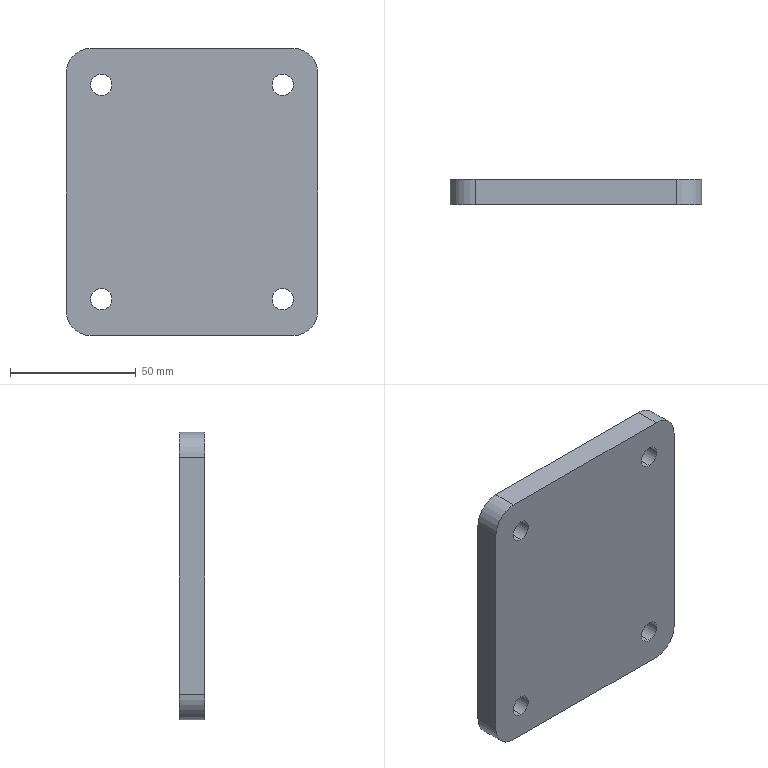Part | SolidWorks | features Extrusion 1, HoleWzd 1 | 1 solid | 18 faces | box 100 x 10 x 114 mm | volume 110872 mm3 | cylinder 12 | plane 6 | commonest cylinder face diameters 8.5 x8 20 x4
STEP:
#1=CARTESIAN_POINT('',(36.,0.,-46.75));
#2=VERTEX_POINT('',#1);
#3=CARTESIAN_POINT('',(36.,0.,-38.25));
#4=VERTEX_POINT('',#3);
#5=CARTESIAN_POINT('',(36.,0.,-42.5));
#6=DIRECTION('',(0.,1.,0.));
#7=DIRECTION('',(0.,0.,1.));
#8=AXIS2_PLACEMENT_3D('',#5,#6,#7);
#9=CIRCLE('',#8,4.25);
#10=EDGE_CURVE('',#2,#4,#9,.T.);
#11=ORIENTED_EDGE('',*,*,#10,.F.);
#12=CARTESIAN_POINT('',(36.,10.,-46.75));
#13=VERTEX_POINT('',#12);
#14=CARTESIAN_POINT('',(36.,10.,-46.75));
#15=DIRECTION('',(0.,1.,0.));
#16=VECTOR('',#15,1000.);
#17=LINE('',#14,#16);
#18=EDGE_CURVE('',#2,#13,#17,.T.);
#19=ORIENTED_EDGE('',*,*,#18,.T.);
#20=CARTESIAN_POINT('',(36.,10.,-38.25));
#21=VERTEX_POINT('',#20);
#22=CARTESIAN_POINT('',(36.,10.,-42.5));
#23=DIRECTION('',(0.,1.,0.));
#24=DIRECTION('',(0.,0.,1.));
#25=AXIS2_PLACEMENT_3D('',#22,#23,#24);
#26=CIRCLE('',#25,4.25);
#27=EDGE_CURVE('',#13,#21,#26,.T.);
#28=ORIENTED_EDGE('',*,*,#27,.T.);
#29=CARTESIAN_POINT('',(36.,10.,-38.25));
#30=DIRECTION('',(0.,1.,0.));
#31=VECTOR('',#30,1000.);
#32=LINE('',#29,#31);
#33=EDGE_CURVE('',#4,#21,#32,.T.);
#34=ORIENTED_EDGE('',*,*,#33,.F.);
#35=EDGE_LOOP('',(#11,#19,#28,#34));
#36=FACE_OUTER_BOUND('',#35,.T.);
#37=CARTESIAN_POINT('',(36.,10.,-42.5));
#38=DIRECTION('',(0.,1.,0.));
#39=DIRECTION('',(0.,0.,1.));
#40=AXIS2_PLACEMENT_3D('',#37,#38,#39);
#41=CYLINDRICAL_SURFACE('',#40,4.25);
#42=ADVANCED_FACE('',(#36),#41,.F.);
#43=CARTESIAN_POINT('',(-36.,0.,38.25));
#44=VERTEX_POINT('',#43);
#45=CARTESIAN_POINT('',(-36.,0.,46.75));
#46=VERTEX_POINT('',#45);
#47=CARTESIAN_POINT('',(-36.,0.,42.5));
#48=DIRECTION('',(0.,1.,0.));
#49=DIRECTION('',(0.,0.,1.));
#50=AXIS2_PLACEMENT_3D('',#47,#48,#49);
#51=CIRCLE('',#50,4.25);
#52=EDGE_CURVE('',#44,#46,#51,.T.);
#53=ORIENTED_EDGE('',*,*,#52,.F.);
#54=CARTESIAN_POINT('',(-36.,10.,38.25));
#55=VERTEX_POINT('',#54);
#56=CARTESIAN_POINT('',(-36.,10.,38.25));
#57=DIRECTION('',(0.,1.,0.));
#58=VECTOR('',#57,1000.);
#59=LINE('',#56,#58);
#60=EDGE_CURVE('',#44,#55,#59,.T.);
#61=ORIENTED_EDGE('',*,*,#60,.T.);
#62=CARTESIAN_POINT('',(-36.,10.,46.75));
#63=VERTEX_POINT('',#62);
#64=CARTESIAN_POINT('',(-36.,10.,42.5));
#65=DIRECTION('',(0.,1.,0.));
#66=DIRECTION('',(0.,0.,1.));
#67=AXIS2_PLACEMENT_3D('',#64,#65,#66);
#68=CIRCLE('',#67,4.25);
#69=EDGE_CURVE('',#55,#63,#68,.T.);
#70=ORIENTED_EDGE('',*,*,#69,.T.);
#71=CARTESIAN_POINT('',(-36.,10.,46.75));
#72=DIRECTION('',(0.,1.,0.));
#73=VECTOR('',#72,1000.);
#74=LINE('',#71,#73);
#75=EDGE_CURVE('',#46,#63,#74,.T.);
#76=ORIENTED_EDGE('',*,*,#75,.F.);
#77=EDGE_LOOP('',(#53,#61,#70,#76));
#78=FACE_OUTER_BOUND('',#77,.T.);
#79=CARTESIAN_POINT('',(-36.,10.,42.5));
#80=DIRECTION('',(0.,1.,0.));
#81=DIRECTION('',(0.,0.,1.));
#82=AXIS2_PLACEMENT_3D('',#79,#80,#81);
#83=CYLINDRICAL_SURFACE('',#82,4.25);
#84=ADVANCED_FACE('',(#78),#83,.F.);
#85=CARTESIAN_POINT('',(-36.,0.,-46.75));
#86=VERTEX_POINT('',#85);
#87=CARTESIAN_POINT('',(-36.,0.,-38.25));
#88=VERTEX_POINT('',#87);
#89=CARTESIAN_POINT('',(-36.,0.,-42.5));
#90=DIRECTION('',(0.,1.,0.));
#91=DIRECTION('',(0.,0.,1.));
#92=AXIS2_PLACEMENT_3D('',#89,#90,#91);
#93=CIRCLE('',#92,4.25);
#94=EDGE_CURVE('',#86,#88,#93,.T.);
#95=ORIENTED_EDGE('',*,*,#94,.F.);
#96=CARTESIAN_POINT('',(-36.,10.,-46.75));
#97=VERTEX_POINT('',#96);
#98=CARTESIAN_POINT('',(-36.,10.,-46.75));
#99=DIRECTION('',(0.,1.,0.));
#100=VECTOR('',#99,1000.);
#101=LINE('',#98,#100);
#102=EDGE_CURVE('',#86,#97,#101,.T.);
#103=ORIENTED_EDGE('',*,*,#102,.T.);
#104=CARTESIAN_POINT('',(-36.,10.,-38.25));
#105=VERTEX_POINT('',#104);
#106=CARTESIAN_POINT('',(-36.,10.,-42.5));
#107=DIRECTION('',(0.,1.,0.));
#108=DIRECTION('',(0.,0.,1.));
#109=AXIS2_PLACEMENT_3D('',#106,#107,#108);
#110=CIRCLE('',#109,4.25);
#111=EDGE_CURVE('',#97,#105,#110,.T.);
#112=ORIENTED_EDGE('',*,*,#111,.T.);
#113=CARTESIAN_POINT('',(-36.,10.,-38.25));
#114=DIRECTION('',(0.,1.,0.));
#115=VECTOR('',#114,1000.);
#116=LINE('',#113,#115);
#117=EDGE_CURVE('',#88,#105,#116,.T.);
#118=ORIENTED_EDGE('',*,*,#117,.F.);
#119=EDGE_LOOP('',(#95,#103,#112,#118));
#120=FACE_OUTER_BOUND('',#119,.T.);
#121=CARTESIAN_POINT('',(-36.,10.,-42.5));
#122=DIRECTION('',(0.,1.,0.));
#123=DIRECTION('',(0.,0.,1.));
#124=AXIS2_PLACEMENT_3D('',#121,#122,#123);
#125=CYLINDRICAL_SURFACE('',#124,4.25);
#126=ADVANCED_FACE('',(#120),#125,.F.);
#127=CARTESIAN_POINT('',(36.,0.,38.25));
#128=VERTEX_POINT('',#127);
#129=CARTESIAN_POINT('',(36.,0.,46.75));
#130=VERTEX_POINT('',#129);
#131=CARTESIAN_POINT('',(36.,0.,42.5));
#132=DIRECTION('',(0.,1.,0.));
#133=DIRECTION('',(0.,0.,1.));
#134=AXIS2_PLACEMENT_3D('',#131,#132,#133);
#135=CIRCLE('',#134,4.25);
#136=EDGE_CURVE('',#128,#130,#135,.T.);
#137=ORIENTED_EDGE('',*,*,#136,.F.);
#138=CARTESIAN_POINT('',(36.,10.,38.25));
#139=VERTEX_POINT('',#138);
#140=CARTESIAN_POINT('',(36.,10.,38.25));
#141=DIRECTION('',(0.,1.,0.));
#142=VECTOR('',#141,1000.);
#143=LINE('',#140,#142);
#144=EDGE_CURVE('',#128,#139,#143,.T.);
#145=ORIENTED_EDGE('',*,*,#144,.T.);
#146=CARTESIAN_POINT('',(36.,10.,46.75));
#147=VERTEX_POINT('',#146);
#148=CARTESIAN_POINT('',(36.,10.,42.5));
#149=DIRECTION('',(0.,1.,0.));
#150=DIRECTION('',(0.,0.,1.));
#151=AXIS2_PLACEMENT_3D('',#148,#149,#150);
#152=CIRCLE('',#151,4.25);
#153=EDGE_CURVE('',#139,#147,#152,.T.);
#154=ORIENTED_EDGE('',*,*,#153,.T.);
#155=CARTESIAN_POINT('',(36.,10.,46.75));
#156=DIRECTION('',(0.,1.,0.));
#157=VECTOR('',#156,1000.);
#158=LINE('',#155,#157);
#159=EDGE_CURVE('',#130,#147,#158,.T.);
#160=ORIENTED_EDGE('',*,*,#159,.F.);
#161=EDGE_LOOP('',(#137,#145,#154,#160));
#162=FACE_OUTER_BOUND('',#161,.T.);
#163=CARTESIAN_POINT('',(36.,10.,42.5));
#164=DIRECTION('',(0.,1.,0.));
#165=DIRECTION('',(0.,0.,1.));
#166=AXIS2_PLACEMENT_3D('',#163,#164,#165);
#167=CYLINDRICAL_SURFACE('',#166,4.25);
#168=ADVANCED_FACE('',(#162),#167,.F.);
#169=CARTESIAN_POINT('',(-50.,0.,47.));
#170=VERTEX_POINT('',#169);
#171=CARTESIAN_POINT('',(-40.,0.,57.));
#172=VERTEX_POINT('',#171);
#173=CARTESIAN_POINT('',(-40.,0.,47.));
#174=DIRECTION('',(0.,1.,0.));
#175=DIRECTION('',(0.,0.,-1.));
#176=AXIS2_PLACEMENT_3D('',#173,#174,#175);
#177=CIRCLE('',#176,10.);
#178=EDGE_CURVE('',#170,#172,#177,.T.);
#179=ORIENTED_EDGE('',*,*,#178,.T.);
#180=CARTESIAN_POINT('',(-40.,10.,57.));
#181=VERTEX_POINT('',#180);
#182=CARTESIAN_POINT('',(-40.,10.,57.));
#183=DIRECTION('',(0.,-1.,0.));
#184=VECTOR('',#183,1000.);
#185=LINE('',#182,#184);
#186=EDGE_CURVE('',#181,#172,#185,.T.);
#187=ORIENTED_EDGE('',*,*,#186,.F.);
#188=CARTESIAN_POINT('',(-50.,10.,47.));
#189=VERTEX_POINT('',#188);
#190=CARTESIAN_POINT('',(-40.,10.,47.));
#191=DIRECTION('',(0.,1.,0.));
#192=DIRECTION('',(0.,0.,-1.));
#193=AXIS2_PLACEMENT_3D('',#190,#191,#192);
#194=CIRCLE('',#193,10.);
#195=EDGE_CURVE('',#189,#181,#194,.T.);
#196=ORIENTED_EDGE('',*,*,#195,.F.);
#197=CARTESIAN_POINT('',(-50.,10.,47.));
#198=DIRECTION('',(0.,-1.,0.));
#199=VECTOR('',#198,1000.);
#200=LINE('',#197,#199);
#201=EDGE_CURVE('',#189,#170,#200,.T.);
#202=ORIENTED_EDGE('',*,*,#201,.T.);
#203=EDGE_LOOP('',(#179,#187,#196,#202));
#204=FACE_OUTER_BOUND('',#203,.T.);
#205=CARTESIAN_POINT('',(-40.,10.,47.));
#206=DIRECTION('',(0.,-1.,0.));
#207=DIRECTION('',(0.,0.,-1.));
#208=AXIS2_PLACEMENT_3D('',#205,#206,#207);
#209=CYLINDRICAL_SURFACE('',#208,10.);
#210=ADVANCED_FACE('',(#204),#209,.T.);
#211=CARTESIAN_POINT('',(40.,0.,57.));
#212=VERTEX_POINT('',#211);
#213=CARTESIAN_POINT('',(-40.,0.,57.));
#214=DIRECTION('',(1.,0.,0.));
#215=VECTOR('',#214,1000.);
#216=LINE('',#213,#215);
#217=EDGE_CURVE('',#172,#212,#216,.T.);
#218=ORIENTED_EDGE('',*,*,#217,.T.);
#219=CARTESIAN_POINT('',(40.,10.,57.));
#220=VERTEX_POINT('',#219);
#221=CARTESIAN_POINT('',(40.,10.,57.));
#222=DIRECTION('',(0.,-1.,0.));
#223=VECTOR('',#222,1000.);
#224=LINE('',#221,#223);
#225=EDGE_CURVE('',#220,#212,#224,.T.);
#226=ORIENTED_EDGE('',*,*,#225,.F.);
#227=CARTESIAN_POINT('',(-40.,10.,57.));
#228=DIRECTION('',(1.,0.,0.));
#229=VECTOR('',#228,1000.);
#230=LINE('',#227,#229);
#231=EDGE_CURVE('',#181,#220,#230,.T.);
#232=ORIENTED_EDGE('',*,*,#231,.F.);
#233=ORIENTED_EDGE('',*,*,#186,.T.);
#234=EDGE_LOOP('',(#218,#226,#232,#233));
#235=FACE_OUTER_BOUND('',#234,.T.);
#236=CARTESIAN_POINT('',(-40.,10.,57.));
#237=DIRECTION('',(0.,0.,-1.));
#238=DIRECTION('',(-1.,0.,0.));
#239=AXIS2_PLACEMENT_3D('',#236,#237,#238);
#240=PLANE('',#239);
#241=ADVANCED_FACE('',(#235),#240,.F.);
#242=CARTESIAN_POINT('',(50.,0.,47.));
#243=VERTEX_POINT('',#242);
#244=CARTESIAN_POINT('',(40.,0.,47.));
#245=DIRECTION('',(0.,1.,0.));
#246=DIRECTION('',(0.,0.,1.));
#247=AXIS2_PLACEMENT_3D('',#244,#245,#246);
#248=CIRCLE('',#247,10.);
#249=EDGE_CURVE('',#212,#243,#248,.T.);
#250=ORIENTED_EDGE('',*,*,#249,.T.);
#251=CARTESIAN_POINT('',(50.,10.,47.));
#252=VERTEX_POINT('',#251);
#253=CARTESIAN_POINT('',(50.,10.,47.));
#254=DIRECTION('',(0.,-1.,0.));
#255=VECTOR('',#254,1000.);
#256=LINE('',#253,#255);
#257=EDGE_CURVE('',#252,#243,#256,.T.);
#258=ORIENTED_EDGE('',*,*,#257,.F.);
#259=CARTESIAN_POINT('',(40.,10.,47.));
#260=DIRECTION('',(0.,1.,0.));
#261=DIRECTION('',(0.,0.,1.));
#262=AXIS2_PLACEMENT_3D('',#259,#260,#261);
#263=CIRCLE('',#262,10.);
#264=EDGE_CURVE('',#220,#252,#263,.T.);
#265=ORIENTED_EDGE('',*,*,#264,.F.);
#266=ORIENTED_EDGE('',*,*,#225,.T.);
#267=EDGE_LOOP('',(#250,#258,#265,#266));
#268=FACE_OUTER_BOUND('',#267,.T.);
#269=CARTESIAN_POINT('',(40.,10.,47.));
#270=DIRECTION('',(0.,-1.,0.));
#271=DIRECTION('',(0.,0.,-1.));
#272=AXIS2_PLACEMENT_3D('',#269,#270,#271);
#273=CYLINDRICAL_SURFACE('',#272,10.);
#274=ADVANCED_FACE('',(#268),#273,.T.);
#275=CARTESIAN_POINT('',(50.,0.,-47.));
#276=VERTEX_POINT('',#275);
#277=CARTESIAN_POINT('',(50.,0.,47.));
#278=DIRECTION('',(0.,0.,-1.));
#279=VECTOR('',#278,1000.);
#280=LINE('',#277,#279);
#281=EDGE_CURVE('',#243,#276,#280,.T.);
#282=ORIENTED_EDGE('',*,*,#281,.T.);
#283=CARTESIAN_POINT('',(50.,10.,-47.));
#284=VERTEX_POINT('',#283);
#285=CARTESIAN_POINT('',(50.,10.,-47.));
#286=DIRECTION('',(0.,-1.,0.));
#287=VECTOR('',#286,1000.);
#288=LINE('',#285,#287);
#289=EDGE_CURVE('',#284,#276,#288,.T.);
#290=ORIENTED_EDGE('',*,*,#289,.F.);
#291=CARTESIAN_POINT('',(50.,10.,47.));
#292=DIRECTION('',(0.,0.,-1.));
#293=VECTOR('',#292,1000.);
#294=LINE('',#291,#293);
#295=EDGE_CURVE('',#252,#284,#294,.T.);
#296=ORIENTED_EDGE('',*,*,#295,.F.);
#297=ORIENTED_EDGE('',*,*,#257,.T.);
#298=EDGE_LOOP('',(#282,#290,#296,#297));
#299=FACE_OUTER_BOUND('',#298,.T.);
#300=CARTESIAN_POINT('',(50.,10.,47.));
#301=DIRECTION('',(-1.,0.,0.));
#302=DIRECTION('',(0.,0.,1.));
#303=AXIS2_PLACEMENT_3D('',#300,#301,#302);
#304=PLANE('',#303);
#305=ADVANCED_FACE('',(#299),#304,.F.);
#306=CARTESIAN_POINT('',(40.,0.,-57.));
#307=VERTEX_POINT('',#306);
#308=CARTESIAN_POINT('',(40.,0.,-47.));
#309=DIRECTION('',(0.,1.,0.));
#310=DIRECTION('',(0.,0.,-1.));
#311=AXIS2_PLACEMENT_3D('',#308,#309,#310);
#312=CIRCLE('',#311,10.);
#313=EDGE_CURVE('',#276,#307,#312,.T.);
#314=ORIENTED_EDGE('',*,*,#313,.T.);
#315=CARTESIAN_POINT('',(40.,10.,-57.));
#316=VERTEX_POINT('',#315);
#317=CARTESIAN_POINT('',(40.,10.,-57.));
#318=DIRECTION('',(0.,-1.,0.));
#319=VECTOR('',#318,1000.);
#320=LINE('',#317,#319);
#321=EDGE_CURVE('',#316,#307,#320,.T.);
#322=ORIENTED_EDGE('',*,*,#321,.F.);
#323=CARTESIAN_POINT('',(40.,10.,-47.));
#324=DIRECTION('',(0.,1.,0.));
#325=DIRECTION('',(0.,0.,-1.));
#326=AXIS2_PLACEMENT_3D('',#323,#324,#325);
#327=CIRCLE('',#326,10.);
#328=EDGE_CURVE('',#284,#316,#327,.T.);
#329=ORIENTED_EDGE('',*,*,#328,.F.);
#330=ORIENTED_EDGE('',*,*,#289,.T.);
#331=EDGE_LOOP('',(#314,#322,#329,#330));
#332=FACE_OUTER_BOUND('',#331,.T.);
#333=CARTESIAN_POINT('',(40.,10.,-47.));
#334=DIRECTION('',(0.,-1.,0.));
#335=DIRECTION('',(0.,0.,-1.));
#336=AXIS2_PLACEMENT_3D('',#333,#334,#335);
#337=CYLINDRICAL_SURFACE('',#336,10.);
#338=ADVANCED_FACE('',(#332),#337,.T.);
#339=CARTESIAN_POINT('',(-40.,0.,-57.));
#340=VERTEX_POINT('',#339);
#341=CARTESIAN_POINT('',(-40.,0.,-57.));
#342=DIRECTION('',(-1.,0.,0.));
#343=VECTOR('',#342,1000.);
#344=LINE('',#341,#343);
#345=EDGE_CURVE('',#307,#340,#344,.T.);
#346=ORIENTED_EDGE('',*,*,#345,.T.);
#347=CARTESIAN_POINT('',(-40.,10.,-57.));
#348=VERTEX_POINT('',#347);
#349=CARTESIAN_POINT('',(-40.,10.,-57.));
#350=DIRECTION('',(0.,-1.,0.));
#351=VECTOR('',#350,1000.);
#352=LINE('',#349,#351);
#353=EDGE_CURVE('',#348,#340,#352,.T.);
#354=ORIENTED_EDGE('',*,*,#353,.F.);
#355=CARTESIAN_POINT('',(-40.,10.,-57.));
#356=DIRECTION('',(-1.,0.,0.));
#357=VECTOR('',#356,1000.);
#358=LINE('',#355,#357);
#359=EDGE_CURVE('',#316,#348,#358,.T.);
#360=ORIENTED_EDGE('',*,*,#359,.F.);
#361=ORIENTED_EDGE('',*,*,#321,.T.);
#362=EDGE_LOOP('',(#346,#354,#360,#361));
#363=FACE_OUTER_BOUND('',#362,.T.);
#364=CARTESIAN_POINT('',(-40.,10.,-57.));
#365=DIRECTION('',(0.,0.,1.));
#366=DIRECTION('',(1.,0.,0.));
#367=AXIS2_PLACEMENT_3D('',#364,#365,#366);
#368=PLANE('',#367);
#369=ADVANCED_FACE('',(#363),#368,.F.);
#370=CARTESIAN_POINT('',(-50.,0.,-47.));
#371=VERTEX_POINT('',#370);
#372=CARTESIAN_POINT('',(-40.,0.,-47.));
#373=DIRECTION('',(0.,1.,0.));
#374=DIRECTION('',(0.,0.,-1.));
#375=AXIS2_PLACEMENT_3D('',#372,#373,#374);
#376=CIRCLE('',#375,10.);
#377=EDGE_CURVE('',#340,#371,#376,.T.);
#378=ORIENTED_EDGE('',*,*,#377,.T.);
#379=CARTESIAN_POINT('',(-50.,10.,-47.));
#380=VERTEX_POINT('',#379);
#381=CARTESIAN_POINT('',(-50.,10.,-47.));
#382=DIRECTION('',(0.,-1.,0.));
#383=VECTOR('',#382,1000.);
#384=LINE('',#381,#383);
#385=EDGE_CURVE('',#380,#371,#384,.T.);
#386=ORIENTED_EDGE('',*,*,#385,.F.);
#387=CARTESIAN_POINT('',(-40.,10.,-47.));
#388=DIRECTION('',(0.,1.,0.));
#389=DIRECTION('',(0.,0.,-1.));
#390=AXIS2_PLACEMENT_3D('',#387,#388,#389);
#391=CIRCLE('',#390,10.);
#392=EDGE_CURVE('',#348,#380,#391,.T.);
#393=ORIENTED_EDGE('',*,*,#392,.F.);
#394=ORIENTED_EDGE('',*,*,#353,.T.);
#395=EDGE_LOOP('',(#378,#386,#393,#394));
#396=FACE_OUTER_BOUND('',#395,.T.);
#397=CARTESIAN_POINT('',(-40.,10.,-47.));
#398=DIRECTION('',(0.,-1.,0.));
#399=DIRECTION('',(0.,0.,-1.));
#400=AXIS2_PLACEMENT_3D('',#397,#398,#399);
#401=CYLINDRICAL_SURFACE('',#400,10.);
#402=ADVANCED_FACE('',(#396),#401,.T.);
#403=CARTESIAN_POINT('',(-50.,0.,47.));
#404=DIRECTION('',(0.,0.,1.));
#405=VECTOR('',#404,1000.);
#406=LINE('',#403,#405);
#407=EDGE_CURVE('',#371,#170,#406,.T.);
#408=ORIENTED_EDGE('',*,*,#407,.T.);
#409=ORIENTED_EDGE('',*,*,#201,.F.);
#410=CARTESIAN_POINT('',(-50.,10.,47.));
#411=DIRECTION('',(0.,0.,1.));
#412=VECTOR('',#411,1000.);
#413=LINE('',#410,#412);
#414=EDGE_CURVE('',#380,#189,#413,.T.);
#415=ORIENTED_EDGE('',*,*,#414,.F.);
#416=ORIENTED_EDGE('',*,*,#385,.T.);
#417=EDGE_LOOP('',(#408,#409,#415,#416));
#418=FACE_OUTER_BOUND('',#417,.T.);
#419=CARTESIAN_POINT('',(-50.,10.,47.));
#420=DIRECTION('',(1.,0.,0.));
#421=DIRECTION('',(0.,0.,-1.));
#422=AXIS2_PLACEMENT_3D('',#419,#420,#421);
#423=PLANE('',#422);
#424=ADVANCED_FACE('',(#418),#423,.F.);
#425=CARTESIAN_POINT('',(36.,10.,-42.5));
#426=DIRECTION('',(0.,1.,0.));
#427=DIRECTION('',(0.,0.,1.));
#428=AXIS2_PLACEMENT_3D('',#425,#426,#427);
#429=CIRCLE('',#428,4.25);
#430=EDGE_CURVE('',#21,#13,#429,.T.);
#431=ORIENTED_EDGE('',*,*,#430,.F.);
#432=ORIENTED_EDGE('',*,*,#27,.F.);
#433=EDGE_LOOP('',(#431,#432));
#434=FACE_BOUND('',#433,.T.);
#435=CARTESIAN_POINT('',(-36.,10.,42.5));
#436=DIRECTION('',(0.,1.,0.));
#437=DIRECTION('',(0.,0.,1.));
#438=AXIS2_PLACEMENT_3D('',#435,#436,#437);
#439=CIRCLE('',#438,4.25);
#440=EDGE_CURVE('',#63,#55,#439,.T.);
#441=ORIENTED_EDGE('',*,*,#440,.F.);
#442=ORIENTED_EDGE('',*,*,#69,.F.);
#443=EDGE_LOOP('',(#441,#442));
#444=FACE_BOUND('',#443,.T.);
#445=CARTESIAN_POINT('',(-36.,10.,-42.5));
#446=DIRECTION('',(0.,1.,0.));
#447=DIRECTION('',(0.,0.,1.));
#448=AXIS2_PLACEMENT_3D('',#445,#446,#447);
#449=CIRCLE('',#448,4.25);
#450=EDGE_CURVE('',#105,#97,#449,.T.);
#451=ORIENTED_EDGE('',*,*,#450,.F.);
#452=ORIENTED_EDGE('',*,*,#111,.F.);
#453=EDGE_LOOP('',(#451,#452));
#454=FACE_BOUND('',#453,.T.);
#455=CARTESIAN_POINT('',(36.,10.,42.5));
#456=DIRECTION('',(0.,1.,0.));
#457=DIRECTION('',(0.,0.,1.));
#458=AXIS2_PLACEMENT_3D('',#455,#456,#457);
#459=CIRCLE('',#458,4.25);
#460=EDGE_CURVE('',#147,#139,#459,.T.);
#461=ORIENTED_EDGE('',*,*,#460,.F.);
#462=ORIENTED_EDGE('',*,*,#153,.F.);
#463=EDGE_LOOP('',(#461,#462));
#464=FACE_BOUND('',#463,.T.);
#465=ORIENTED_EDGE('',*,*,#195,.T.);
#466=ORIENTED_EDGE('',*,*,#231,.T.);
#467=ORIENTED_EDGE('',*,*,#264,.T.);
#468=ORIENTED_EDGE('',*,*,#295,.T.);
#469=ORIENTED_EDGE('',*,*,#328,.T.);
#470=ORIENTED_EDGE('',*,*,#359,.T.);
#471=ORIENTED_EDGE('',*,*,#392,.T.);
#472=ORIENTED_EDGE('',*,*,#414,.T.);
#473=EDGE_LOOP('',(#465,#466,#467,#468,#469,#470,#471,#472));
#474=FACE_OUTER_BOUND('',#473,.T.);
#475=CARTESIAN_POINT('',(-40.,10.,47.));
#476=DIRECTION('',(0.,-1.,0.));
#477=DIRECTION('',(0.,0.,-1.));
#478=AXIS2_PLACEMENT_3D('',#475,#476,#477);
#479=PLANE('',#478);
#480=ADVANCED_FACE('',(#434,#444,#454,#464,#474),#479,.F.);
#481=CARTESIAN_POINT('',(36.,0.,-42.5));
#482=DIRECTION('',(0.,1.,0.));
#483=DIRECTION('',(0.,0.,1.));
#484=AXIS2_PLACEMENT_3D('',#481,#482,#483);
#485=CIRCLE('',#484,4.25);
#486=EDGE_CURVE('',#4,#2,#485,.T.);
#487=ORIENTED_EDGE('',*,*,#486,.T.);
#488=ORIENTED_EDGE('',*,*,#10,.T.);
#489=EDGE_LOOP('',(#487,#488));
#490=FACE_BOUND('',#489,.T.);
#491=CARTESIAN_POINT('',(-36.,0.,42.5));
#492=DIRECTION('',(0.,1.,0.));
#493=DIRECTION('',(0.,0.,1.));
#494=AXIS2_PLACEMENT_3D('',#491,#492,#493);
#495=CIRCLE('',#494,4.25);
#496=EDGE_CURVE('',#46,#44,#495,.T.);
#497=ORIENTED_EDGE('',*,*,#496,.T.);
#498=ORIENTED_EDGE('',*,*,#52,.T.);
#499=EDGE_LOOP('',(#497,#498));
#500=FACE_BOUND('',#499,.T.);
#501=CARTESIAN_POINT('',(-36.,0.,-42.5));
#502=DIRECTION('',(0.,1.,0.));
#503=DIRECTION('',(0.,0.,1.));
#504=AXIS2_PLACEMENT_3D('',#501,#502,#503);
#505=CIRCLE('',#504,4.25);
#506=EDGE_CURVE('',#88,#86,#505,.T.);
#507=ORIENTED_EDGE('',*,*,#506,.T.);
#508=ORIENTED_EDGE('',*,*,#94,.T.);
#509=EDGE_LOOP('',(#507,#508));
#510=FACE_BOUND('',#509,.T.);
#511=CARTESIAN_POINT('',(36.,0.,42.5));
#512=DIRECTION('',(0.,1.,0.));
#513=DIRECTION('',(0.,0.,1.));
#514=AXIS2_PLACEMENT_3D('',#511,#512,#513);
#515=CIRCLE('',#514,4.25);
#516=EDGE_CURVE('',#130,#128,#515,.T.);
#517=ORIENTED_EDGE('',*,*,#516,.T.);
#518=ORIENTED_EDGE('',*,*,#136,.T.);
#519=EDGE_LOOP('',(#517,#518));
#520=FACE_BOUND('',#519,.T.);
#521=ORIENTED_EDGE('',*,*,#178,.F.);
#522=ORIENTED_EDGE('',*,*,#407,.F.);
#523=ORIENTED_EDGE('',*,*,#377,.F.);
#524=ORIENTED_EDGE('',*,*,#345,.F.);
#525=ORIENTED_EDGE('',*,*,#313,.F.);
#526=ORIENTED_EDGE('',*,*,#281,.F.);
#527=ORIENTED_EDGE('',*,*,#249,.F.);
#528=ORIENTED_EDGE('',*,*,#217,.F.);
#529=EDGE_LOOP('',(#521,#522,#523,#524,#525,#526,#527,#528));
#530=FACE_OUTER_BOUND('',#529,.T.);
#531=CARTESIAN_POINT('',(-40.,0.,47.));
#532=DIRECTION('',(0.,-1.,0.));
#533=DIRECTION('',(0.,0.,-1.));
#534=AXIS2_PLACEMENT_3D('',#531,#532,#533);
#535=PLANE('',#534);
#536=ADVANCED_FACE('',(#490,#500,#510,#520,#530),#535,.T.);
#537=ORIENTED_EDGE('',*,*,#144,.F.);
#538=ORIENTED_EDGE('',*,*,#516,.F.);
#539=ORIENTED_EDGE('',*,*,#159,.T.);
#540=ORIENTED_EDGE('',*,*,#460,.T.);
#541=EDGE_LOOP('',(#537,#538,#539,#540));
#542=FACE_OUTER_BOUND('',#541,.T.);
#543=CARTESIAN_POINT('',(36.,10.,42.5));
#544=DIRECTION('',(0.,1.,0.));
#545=DIRECTION('',(0.,0.,1.));
#546=AXIS2_PLACEMENT_3D('',#543,#544,#545);
#547=CYLINDRICAL_SURFACE('',#546,4.25);
#548=ADVANCED_FACE('',(#542),#547,.F.);
#549=ORIENTED_EDGE('',*,*,#102,.F.);
#550=ORIENTED_EDGE('',*,*,#506,.F.);
#551=ORIENTED_EDGE('',*,*,#117,.T.);
#552=ORIENTED_EDGE('',*,*,#450,.T.);
#553=EDGE_LOOP('',(#549,#550,#551,#552));
#554=FACE_OUTER_BOUND('',#553,.T.);
#555=CARTESIAN_POINT('',(-36.,10.,-42.5));
#556=DIRECTION('',(0.,1.,0.));
#557=DIRECTION('',(0.,0.,1.));
#558=AXIS2_PLACEMENT_3D('',#555,#556,#557);
#559=CYLINDRICAL_SURFACE('',#558,4.25);
#560=ADVANCED_FACE('',(#554),#559,.F.);
#561=ORIENTED_EDGE('',*,*,#60,.F.);
#562=ORIENTED_EDGE('',*,*,#496,.F.);
#563=ORIENTED_EDGE('',*,*,#75,.T.);
#564=ORIENTED_EDGE('',*,*,#440,.T.);
#565=EDGE_LOOP('',(#561,#562,#563,#564));
#566=FACE_OUTER_BOUND('',#565,.T.);
#567=CARTESIAN_POINT('',(-36.,10.,42.5));
#568=DIRECTION('',(0.,1.,0.));
#569=DIRECTION('',(0.,0.,1.));
#570=AXIS2_PLACEMENT_3D('',#567,#568,#569);
#571=CYLINDRICAL_SURFACE('',#570,4.25);
#572=ADVANCED_FACE('',(#566),#571,.F.);
#573=ORIENTED_EDGE('',*,*,#18,.F.);
#574=ORIENTED_EDGE('',*,*,#486,.F.);
#575=ORIENTED_EDGE('',*,*,#33,.T.);
#576=ORIENTED_EDGE('',*,*,#430,.T.);
#577=EDGE_LOOP('',(#573,#574,#575,#576));
#578=FACE_OUTER_BOUND('',#577,.T.);
#579=CARTESIAN_POINT('',(36.,10.,-42.5));
#580=DIRECTION('',(0.,1.,0.));
#581=DIRECTION('',(0.,0.,1.));
#582=AXIS2_PLACEMENT_3D('',#579,#580,#581);
#583=CYLINDRICAL_SURFACE('',#582,4.25);
#584=ADVANCED_FACE('',(#578),#583,.F.);
#585=CLOSED_SHELL('',(#42,#84,#126,#168,#210,#241,#274,#305,#338,#369,#402,#424,#480,#536,#548,#560,#572,#584));
#586=MANIFOLD_SOLID_BREP('',#585);
#587=CARTESIAN_POINT('',(0.,0.,0.));
#588=DIRECTION('',(0.,0.,1.));
#589=DIRECTION('',(1.,0.,0.));
#590=AXIS2_PLACEMENT_3D('',#587,#588,#589);
#591=(LENGTH_UNIT()NAMED_UNIT(*)SI_UNIT(.MILLI.,.METRE.));
#592=UNCERTAINTY_MEASURE_WITH_UNIT(LENGTH_MEASURE(0.00001),#591,'','');
#593=(NAMED_UNIT(*)PLANE_ANGLE_UNIT()SI_UNIT($,.RADIAN.));
#594=(NAMED_UNIT(*)SI_UNIT($,.STERADIAN.)SOLID_ANGLE_UNIT());
#595=(GEOMETRIC_REPRESENTATION_CONTEXT(3)GLOBAL_UNCERTAINTY_ASSIGNED_CONTEXT((#592))GLOBAL_UNIT_ASSIGNED_CONTEXT((#591,#593,#594))REPRESENTATION_CONTEXT('',''));
#596=ADVANCED_BREP_SHAPE_REPRESENTATION('',(#586,#590),#595);